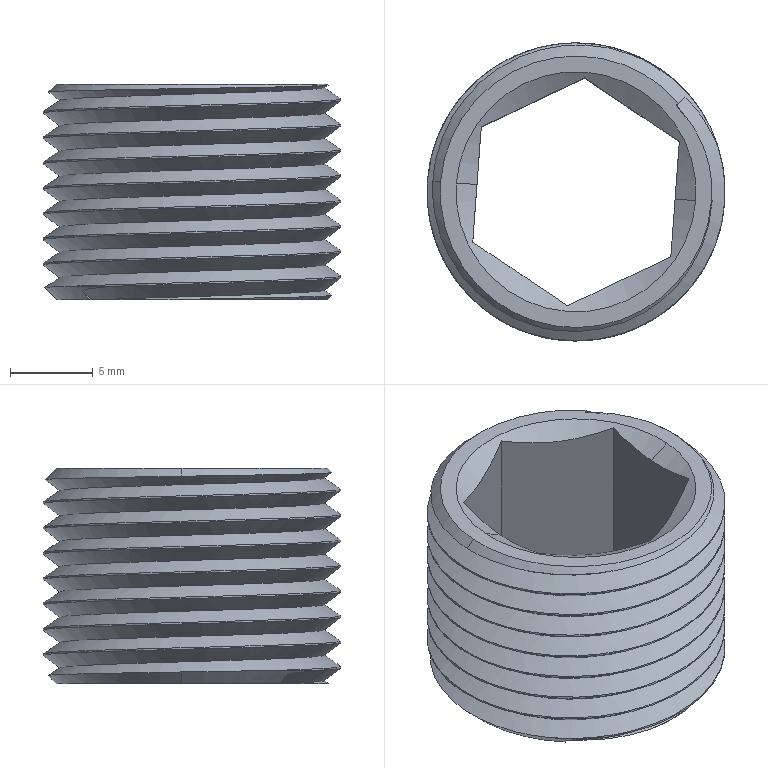Part | SolidWorks | features BaseBody 1 | 1 solid | 42 faces | box 18 x 18 x 13 mm | volume 1327 mm3 | cylinder 16 | plane 16 | cone 8 | spline 2 | commonest cylinder face diameters 18 x16